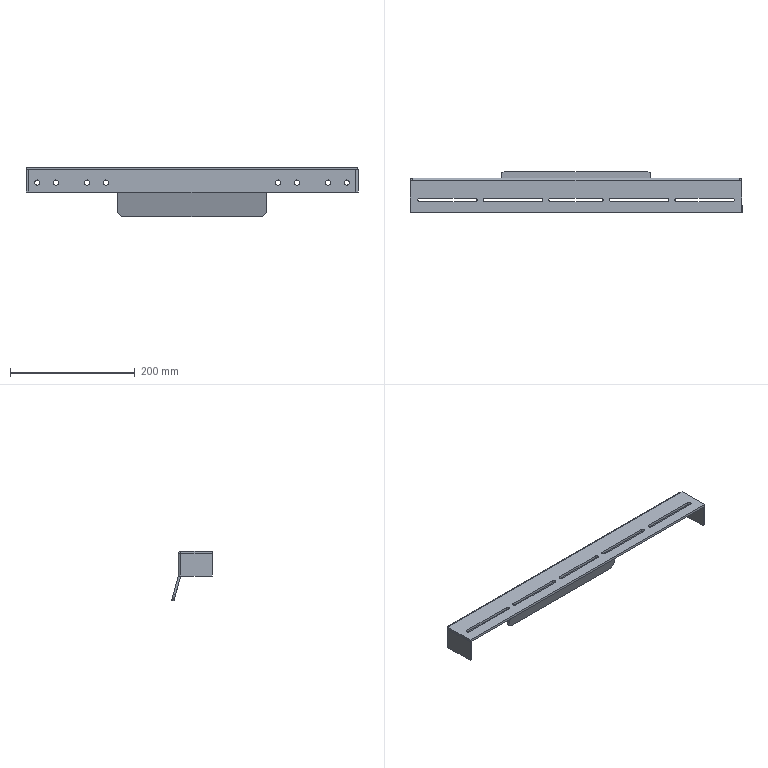Part | SolidWorks | features ICE 3, EdgeFlange 2, Fillet 1, FlatPattern 1, SMBaseFlange 1, SheetMetal 1 | 1 solid | 82 faces | box 532 x 65.443 x 80 mm | volume 231503 mm3 | plane 43 | cylinder 39 | commonest cylinder face diameters 8.5 x16 6 x15 0.2 x3 8.2 x3 20 x2